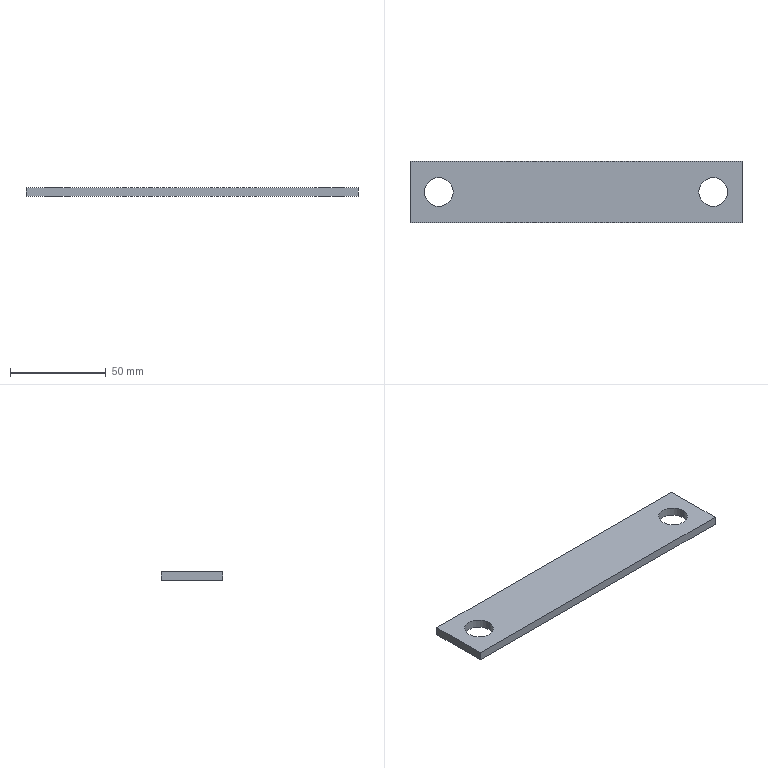Part | SolidWorks | features FlatPattern 1, SMBaseFlange 1, SheetMetal 1 | 1 solid | 10 faces | box 173 x 32 x 4.5 mm | volume 23322 mm3 | plane 6 | cylinder 4 | commonest cylinder face diameters 15 x4
STEP:
#1=CARTESIAN_POINT('',(64.,0.,-4.5));
#2=VERTEX_POINT('',#1);
#3=CARTESIAN_POINT('',(79.,0.,-4.5));
#4=VERTEX_POINT('',#3);
#5=CARTESIAN_POINT('',(71.5,0.,-4.5));
#6=DIRECTION('',(0.,0.,1.));
#7=DIRECTION('',(1.,0.,0.));
#8=AXIS2_PLACEMENT_3D('',#5,#6,#7);
#9=CIRCLE('',#8,7.5);
#10=EDGE_CURVE('',#2,#4,#9,.T.);
#11=ORIENTED_EDGE('',*,*,#10,.F.);
#12=CARTESIAN_POINT('',(64.,0.,0.));
#13=VERTEX_POINT('',#12);
#14=CARTESIAN_POINT('',(64.,0.,-4.5));
#15=DIRECTION('',(0.,0.,1.));
#16=VECTOR('',#15,1000.);
#17=LINE('',#14,#16);
#18=EDGE_CURVE('',#2,#13,#17,.T.);
#19=ORIENTED_EDGE('',*,*,#18,.T.);
#20=CARTESIAN_POINT('',(79.,0.,0.));
#21=VERTEX_POINT('',#20);
#22=CARTESIAN_POINT('',(71.5,0.,0.));
#23=DIRECTION('',(0.,0.,1.));
#24=DIRECTION('',(1.,0.,0.));
#25=AXIS2_PLACEMENT_3D('',#22,#23,#24);
#26=CIRCLE('',#25,7.5);
#27=EDGE_CURVE('',#13,#21,#26,.T.);
#28=ORIENTED_EDGE('',*,*,#27,.T.);
#29=CARTESIAN_POINT('',(79.,0.,-4.5));
#30=DIRECTION('',(0.,0.,1.));
#31=VECTOR('',#30,1000.);
#32=LINE('',#29,#31);
#33=EDGE_CURVE('',#4,#21,#32,.T.);
#34=ORIENTED_EDGE('',*,*,#33,.F.);
#35=EDGE_LOOP('',(#11,#19,#28,#34));
#36=FACE_OUTER_BOUND('',#35,.T.);
#37=CARTESIAN_POINT('',(71.5,0.,-4.5));
#38=DIRECTION('',(0.,0.,1.));
#39=DIRECTION('',(1.,0.,0.));
#40=AXIS2_PLACEMENT_3D('',#37,#38,#39);
#41=CYLINDRICAL_SURFACE('',#40,7.5);
#42=ADVANCED_FACE('',(#36),#41,.F.);
#43=CARTESIAN_POINT('',(-79.,0.,-4.5));
#44=VERTEX_POINT('',#43);
#45=CARTESIAN_POINT('',(-64.,0.,-4.5));
#46=VERTEX_POINT('',#45);
#47=CARTESIAN_POINT('',(-71.5,0.,-4.5));
#48=DIRECTION('',(0.,0.,1.));
#49=DIRECTION('',(1.,0.,0.));
#50=AXIS2_PLACEMENT_3D('',#47,#48,#49);
#51=CIRCLE('',#50,7.5);
#52=EDGE_CURVE('',#44,#46,#51,.T.);
#53=ORIENTED_EDGE('',*,*,#52,.F.);
#54=CARTESIAN_POINT('',(-79.,0.,0.));
#55=VERTEX_POINT('',#54);
#56=CARTESIAN_POINT('',(-79.,0.,-4.5));
#57=DIRECTION('',(0.,0.,1.));
#58=VECTOR('',#57,1000.);
#59=LINE('',#56,#58);
#60=EDGE_CURVE('',#44,#55,#59,.T.);
#61=ORIENTED_EDGE('',*,*,#60,.T.);
#62=CARTESIAN_POINT('',(-64.,0.,0.));
#63=VERTEX_POINT('',#62);
#64=CARTESIAN_POINT('',(-71.5,0.,0.));
#65=DIRECTION('',(0.,0.,1.));
#66=DIRECTION('',(1.,0.,0.));
#67=AXIS2_PLACEMENT_3D('',#64,#65,#66);
#68=CIRCLE('',#67,7.5);
#69=EDGE_CURVE('',#55,#63,#68,.T.);
#70=ORIENTED_EDGE('',*,*,#69,.T.);
#71=CARTESIAN_POINT('',(-64.,0.,-4.5));
#72=DIRECTION('',(0.,0.,1.));
#73=VECTOR('',#72,1000.);
#74=LINE('',#71,#73);
#75=EDGE_CURVE('',#46,#63,#74,.T.);
#76=ORIENTED_EDGE('',*,*,#75,.F.);
#77=EDGE_LOOP('',(#53,#61,#70,#76));
#78=FACE_OUTER_BOUND('',#77,.T.);
#79=CARTESIAN_POINT('',(-71.5,0.,-4.5));
#80=DIRECTION('',(0.,0.,1.));
#81=DIRECTION('',(1.,0.,0.));
#82=AXIS2_PLACEMENT_3D('',#79,#80,#81);
#83=CYLINDRICAL_SURFACE('',#82,7.5);
#84=ADVANCED_FACE('',(#78),#83,.F.);
#85=CARTESIAN_POINT('',(86.5,-16.,0.));
#86=VERTEX_POINT('',#85);
#87=CARTESIAN_POINT('',(86.5,16.,0.));
#88=VERTEX_POINT('',#87);
#89=CARTESIAN_POINT('',(86.5,16.,0.));
#90=DIRECTION('',(0.,1.,0.));
#91=VECTOR('',#90,1000.);
#92=LINE('',#89,#91);
#93=EDGE_CURVE('',#86,#88,#92,.T.);
#94=ORIENTED_EDGE('',*,*,#93,.F.);
#95=CARTESIAN_POINT('',(86.5,-16.,-4.5));
#96=VERTEX_POINT('',#95);
#97=CARTESIAN_POINT('',(86.5,-16.,-4.5));
#98=DIRECTION('',(0.,0.,1.));
#99=VECTOR('',#98,1000.);
#100=LINE('',#97,#99);
#101=EDGE_CURVE('',#96,#86,#100,.T.);
#102=ORIENTED_EDGE('',*,*,#101,.F.);
#103=CARTESIAN_POINT('',(86.5,16.,-4.5));
#104=VERTEX_POINT('',#103);
#105=CARTESIAN_POINT('',(86.5,16.,-4.5));
#106=DIRECTION('',(0.,1.,0.));
#107=VECTOR('',#106,1000.);
#108=LINE('',#105,#107);
#109=EDGE_CURVE('',#96,#104,#108,.T.);
#110=ORIENTED_EDGE('',*,*,#109,.T.);
#111=CARTESIAN_POINT('',(86.5,16.,-4.5));
#112=DIRECTION('',(0.,0.,1.));
#113=VECTOR('',#112,1000.);
#114=LINE('',#111,#113);
#115=EDGE_CURVE('',#104,#88,#114,.T.);
#116=ORIENTED_EDGE('',*,*,#115,.T.);
#117=EDGE_LOOP('',(#94,#102,#110,#116));
#118=FACE_OUTER_BOUND('',#117,.T.);
#119=CARTESIAN_POINT('',(86.5,16.,-4.5));
#120=DIRECTION('',(1.,0.,0.));
#121=DIRECTION('',(0.,0.,-1.));
#122=AXIS2_PLACEMENT_3D('',#119,#120,#121);
#123=PLANE('',#122);
#124=ADVANCED_FACE('',(#118),#123,.T.);
#125=CARTESIAN_POINT('',(-86.5,-16.,0.));
#126=VERTEX_POINT('',#125);
#127=CARTESIAN_POINT('',(-86.5,-16.,0.));
#128=DIRECTION('',(1.,0.,0.));
#129=VECTOR('',#128,1000.);
#130=LINE('',#127,#129);
#131=EDGE_CURVE('',#126,#86,#130,.T.);
#132=ORIENTED_EDGE('',*,*,#131,.F.);
#133=CARTESIAN_POINT('',(-86.5,-16.,-4.5));
#134=VERTEX_POINT('',#133);
#135=CARTESIAN_POINT('',(-86.5,-16.,-4.5));
#136=DIRECTION('',(0.,0.,1.));
#137=VECTOR('',#136,1000.);
#138=LINE('',#135,#137);
#139=EDGE_CURVE('',#134,#126,#138,.T.);
#140=ORIENTED_EDGE('',*,*,#139,.F.);
#141=CARTESIAN_POINT('',(-86.5,-16.,-4.5));
#142=DIRECTION('',(1.,0.,0.));
#143=VECTOR('',#142,1000.);
#144=LINE('',#141,#143);
#145=EDGE_CURVE('',#134,#96,#144,.T.);
#146=ORIENTED_EDGE('',*,*,#145,.T.);
#147=ORIENTED_EDGE('',*,*,#101,.T.);
#148=EDGE_LOOP('',(#132,#140,#146,#147));
#149=FACE_OUTER_BOUND('',#148,.T.);
#150=CARTESIAN_POINT('',(-86.5,-16.,-4.5));
#151=DIRECTION('',(0.,-1.,0.));
#152=DIRECTION('',(0.,0.,-1.));
#153=AXIS2_PLACEMENT_3D('',#150,#151,#152);
#154=PLANE('',#153);
#155=ADVANCED_FACE('',(#149),#154,.T.);
#156=CARTESIAN_POINT('',(-86.5,16.,0.));
#157=VERTEX_POINT('',#156);
#158=CARTESIAN_POINT('',(-86.5,16.,0.));
#159=DIRECTION('',(0.,-1.,0.));
#160=VECTOR('',#159,1000.);
#161=LINE('',#158,#160);
#162=EDGE_CURVE('',#157,#126,#161,.T.);
#163=ORIENTED_EDGE('',*,*,#162,.F.);
#164=CARTESIAN_POINT('',(-86.5,16.,-4.5));
#165=VERTEX_POINT('',#164);
#166=CARTESIAN_POINT('',(-86.5,16.,-4.5));
#167=DIRECTION('',(0.,0.,1.));
#168=VECTOR('',#167,1000.);
#169=LINE('',#166,#168);
#170=EDGE_CURVE('',#165,#157,#169,.T.);
#171=ORIENTED_EDGE('',*,*,#170,.F.);
#172=CARTESIAN_POINT('',(-86.5,16.,-4.5));
#173=DIRECTION('',(0.,-1.,0.));
#174=VECTOR('',#173,1000.);
#175=LINE('',#172,#174);
#176=EDGE_CURVE('',#165,#134,#175,.T.);
#177=ORIENTED_EDGE('',*,*,#176,.T.);
#178=ORIENTED_EDGE('',*,*,#139,.T.);
#179=EDGE_LOOP('',(#163,#171,#177,#178));
#180=FACE_OUTER_BOUND('',#179,.T.);
#181=CARTESIAN_POINT('',(-86.5,16.,-4.5));
#182=DIRECTION('',(-1.,0.,0.));
#183=DIRECTION('',(0.,0.,1.));
#184=AXIS2_PLACEMENT_3D('',#181,#182,#183);
#185=PLANE('',#184);
#186=ADVANCED_FACE('',(#180),#185,.T.);
#187=CARTESIAN_POINT('',(-86.5,16.,0.));
#188=DIRECTION('',(-1.,0.,0.));
#189=VECTOR('',#188,1000.);
#190=LINE('',#187,#189);
#191=EDGE_CURVE('',#88,#157,#190,.T.);
#192=ORIENTED_EDGE('',*,*,#191,.F.);
#193=ORIENTED_EDGE('',*,*,#115,.F.);
#194=CARTESIAN_POINT('',(-86.5,16.,-4.5));
#195=DIRECTION('',(-1.,0.,0.));
#196=VECTOR('',#195,1000.);
#197=LINE('',#194,#196);
#198=EDGE_CURVE('',#104,#165,#197,.T.);
#199=ORIENTED_EDGE('',*,*,#198,.T.);
#200=ORIENTED_EDGE('',*,*,#170,.T.);
#201=EDGE_LOOP('',(#192,#193,#199,#200));
#202=FACE_OUTER_BOUND('',#201,.T.);
#203=CARTESIAN_POINT('',(-86.5,16.,-4.5));
#204=DIRECTION('',(0.,1.,0.));
#205=DIRECTION('',(0.,0.,1.));
#206=AXIS2_PLACEMENT_3D('',#203,#204,#205);
#207=PLANE('',#206);
#208=ADVANCED_FACE('',(#202),#207,.T.);
#209=CARTESIAN_POINT('',(71.5,0.,-4.5));
#210=DIRECTION('',(0.,0.,1.));
#211=DIRECTION('',(1.,0.,0.));
#212=AXIS2_PLACEMENT_3D('',#209,#210,#211);
#213=CIRCLE('',#212,7.5);
#214=EDGE_CURVE('',#4,#2,#213,.T.);
#215=ORIENTED_EDGE('',*,*,#214,.T.);
#216=ORIENTED_EDGE('',*,*,#10,.T.);
#217=EDGE_LOOP('',(#215,#216));
#218=FACE_BOUND('',#217,.T.);
#219=CARTESIAN_POINT('',(-71.5,0.,-4.5));
#220=DIRECTION('',(0.,0.,1.));
#221=DIRECTION('',(1.,0.,0.));
#222=AXIS2_PLACEMENT_3D('',#219,#220,#221);
#223=CIRCLE('',#222,7.5);
#224=EDGE_CURVE('',#46,#44,#223,.T.);
#225=ORIENTED_EDGE('',*,*,#224,.T.);
#226=ORIENTED_EDGE('',*,*,#52,.T.);
#227=EDGE_LOOP('',(#225,#226));
#228=FACE_BOUND('',#227,.T.);
#229=ORIENTED_EDGE('',*,*,#109,.F.);
#230=ORIENTED_EDGE('',*,*,#145,.F.);
#231=ORIENTED_EDGE('',*,*,#176,.F.);
#232=ORIENTED_EDGE('',*,*,#198,.F.);
#233=EDGE_LOOP('',(#229,#230,#231,#232));
#234=FACE_OUTER_BOUND('',#233,.T.);
#235=CARTESIAN_POINT('',(0.,0.,-4.5));
#236=DIRECTION('',(0.,0.,1.));
#237=DIRECTION('',(1.,0.,0.));
#238=AXIS2_PLACEMENT_3D('',#235,#236,#237);
#239=PLANE('',#238);
#240=ADVANCED_FACE('',(#218,#228,#234),#239,.F.);
#241=CARTESIAN_POINT('',(71.5,0.,0.));
#242=DIRECTION('',(0.,0.,1.));
#243=DIRECTION('',(1.,0.,0.));
#244=AXIS2_PLACEMENT_3D('',#241,#242,#243);
#245=CIRCLE('',#244,7.5);
#246=EDGE_CURVE('',#21,#13,#245,.T.);
#247=ORIENTED_EDGE('',*,*,#246,.F.);
#248=ORIENTED_EDGE('',*,*,#27,.F.);
#249=EDGE_LOOP('',(#247,#248));
#250=FACE_BOUND('',#249,.T.);
#251=CARTESIAN_POINT('',(-71.5,0.,0.));
#252=DIRECTION('',(0.,0.,1.));
#253=DIRECTION('',(1.,0.,0.));
#254=AXIS2_PLACEMENT_3D('',#251,#252,#253);
#255=CIRCLE('',#254,7.5);
#256=EDGE_CURVE('',#63,#55,#255,.T.);
#257=ORIENTED_EDGE('',*,*,#256,.F.);
#258=ORIENTED_EDGE('',*,*,#69,.F.);
#259=EDGE_LOOP('',(#257,#258));
#260=FACE_BOUND('',#259,.T.);
#261=ORIENTED_EDGE('',*,*,#93,.T.);
#262=ORIENTED_EDGE('',*,*,#191,.T.);
#263=ORIENTED_EDGE('',*,*,#162,.T.);
#264=ORIENTED_EDGE('',*,*,#131,.T.);
#265=EDGE_LOOP('',(#261,#262,#263,#264));
#266=FACE_OUTER_BOUND('',#265,.T.);
#267=CARTESIAN_POINT('',(0.,0.,0.));
#268=DIRECTION('',(0.,0.,1.));
#269=DIRECTION('',(1.,0.,0.));
#270=AXIS2_PLACEMENT_3D('',#267,#268,#269);
#271=PLANE('',#270);
#272=ADVANCED_FACE('',(#250,#260,#266),#271,.T.);
#273=ORIENTED_EDGE('',*,*,#60,.F.);
#274=ORIENTED_EDGE('',*,*,#224,.F.);
#275=ORIENTED_EDGE('',*,*,#75,.T.);
#276=ORIENTED_EDGE('',*,*,#256,.T.);
#277=EDGE_LOOP('',(#273,#274,#275,#276));
#278=FACE_OUTER_BOUND('',#277,.T.);
#279=CARTESIAN_POINT('',(-71.5,0.,-4.5));
#280=DIRECTION('',(0.,0.,1.));
#281=DIRECTION('',(1.,0.,0.));
#282=AXIS2_PLACEMENT_3D('',#279,#280,#281);
#283=CYLINDRICAL_SURFACE('',#282,7.5);
#284=ADVANCED_FACE('',(#278),#283,.F.);
#285=ORIENTED_EDGE('',*,*,#18,.F.);
#286=ORIENTED_EDGE('',*,*,#214,.F.);
#287=ORIENTED_EDGE('',*,*,#33,.T.);
#288=ORIENTED_EDGE('',*,*,#246,.T.);
#289=EDGE_LOOP('',(#285,#286,#287,#288));
#290=FACE_OUTER_BOUND('',#289,.T.);
#291=CARTESIAN_POINT('',(71.5,0.,-4.5));
#292=DIRECTION('',(0.,0.,1.));
#293=DIRECTION('',(1.,0.,0.));
#294=AXIS2_PLACEMENT_3D('',#291,#292,#293);
#295=CYLINDRICAL_SURFACE('',#294,7.5);
#296=ADVANCED_FACE('',(#290),#295,.F.);
#297=CLOSED_SHELL('',(#42,#84,#124,#155,#186,#208,#240,#272,#284,#296));
#298=MANIFOLD_SOLID_BREP('',#297);
#299=CARTESIAN_POINT('',(0.,0.,0.));
#300=DIRECTION('',(0.,0.,1.));
#301=DIRECTION('',(1.,0.,0.));
#302=AXIS2_PLACEMENT_3D('',#299,#300,#301);
#303=(LENGTH_UNIT()NAMED_UNIT(*)SI_UNIT(.MILLI.,.METRE.));
#304=UNCERTAINTY_MEASURE_WITH_UNIT(LENGTH_MEASURE(0.00001),#303,'','');
#305=(NAMED_UNIT(*)PLANE_ANGLE_UNIT()SI_UNIT($,.RADIAN.));
#306=(NAMED_UNIT(*)SI_UNIT($,.STERADIAN.)SOLID_ANGLE_UNIT());
#307=(GEOMETRIC_REPRESENTATION_CONTEXT(3)GLOBAL_UNCERTAINTY_ASSIGNED_CONTEXT((#304))GLOBAL_UNIT_ASSIGNED_CONTEXT((#303,#305,#306))REPRESENTATION_CONTEXT('',''));
#308=ADVANCED_BREP_SHAPE_REPRESENTATION('',(#298,#302),#307);